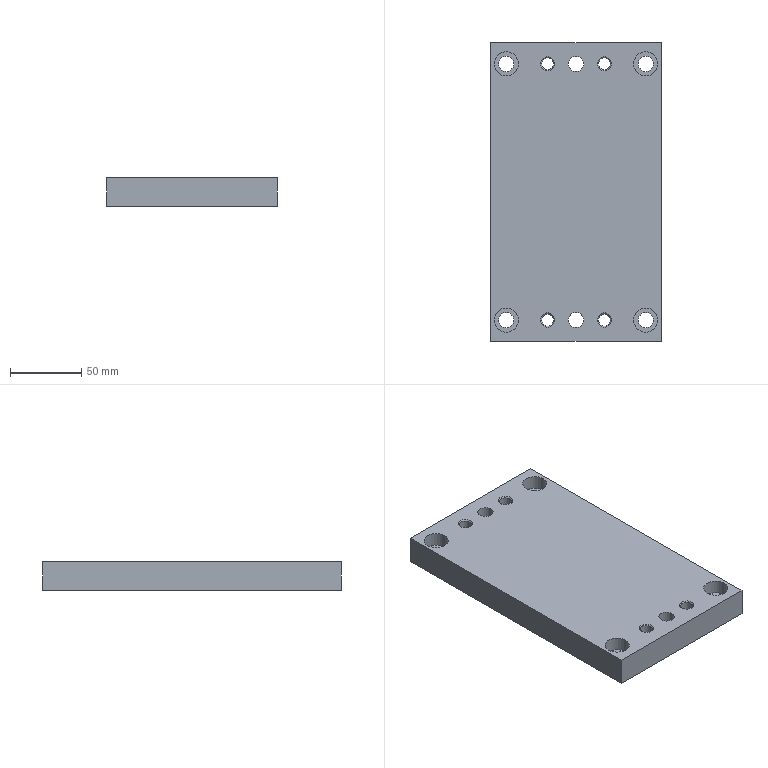Part | STEP file | YBQDJ-YB-4 | 1 solid | 32 faces | box 120 x 210 x 20 mm | volume 483124 mm3 | cylinder 14 | plane 10 | cone 8 | commonest cylinder face diameters 10.7 x6 8.5 x4 17 x4